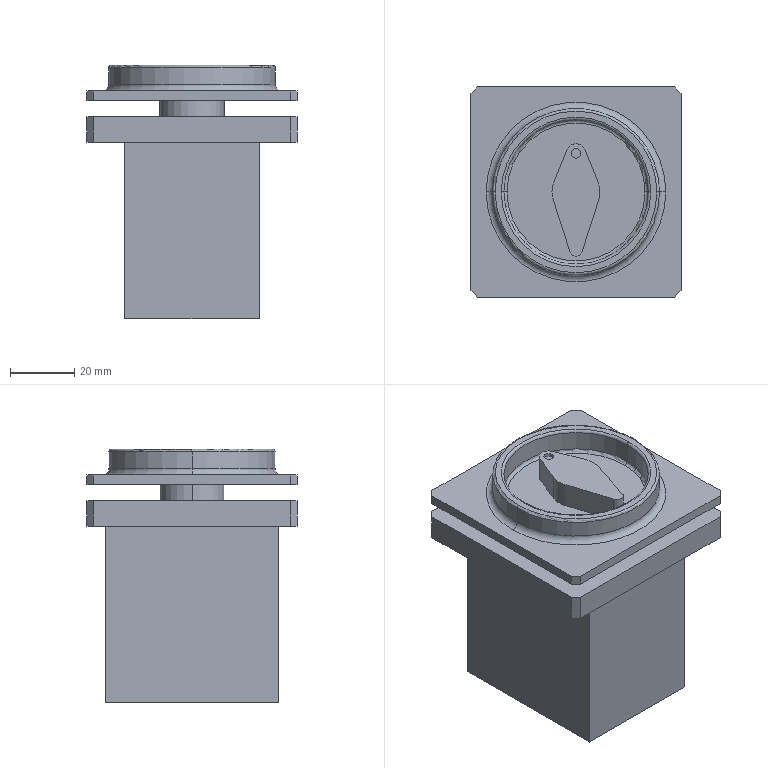Part | SolidWorks | features ICE 6, Fillet 3, Chamfer 2, Extrusion 1, HoleWzd 1 | 1 solid | 62 faces | box 65.5 x 65.5 x 79 mm | volume 180207 mm3 | plane 33 | cylinder 21 | torus 8 | commonest cylinder face diameters 3.3 x8 15 x3 3 x2 20 x2 45 x2 52 x2